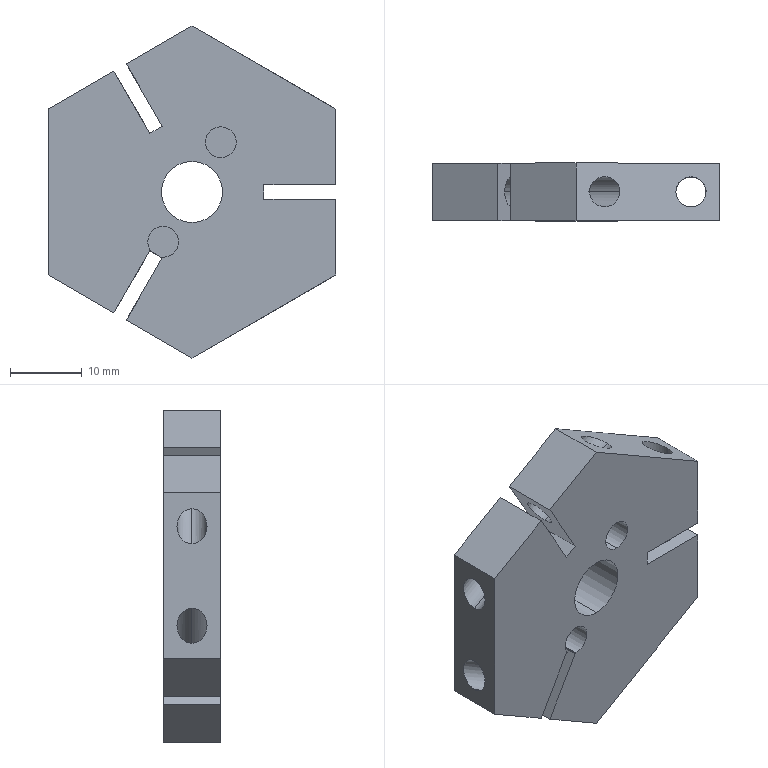Part | SolidWorks | features ICE 3, CirPattern 2, Cut 1, Extrusion 1 | 1 solid | 41 faces | box 40 x 8 x 46.188 mm | volume 8880 mm3 | plane 22 | cylinder 19 | commonest cylinder face diameters 4.2 x12 4.3 x5 8.5 x2
STEP:
#1=CARTESIAN_POINT('',(-4.,0.,-9.078));
#2=VERTEX_POINT('',#1);
#3=CARTESIAN_POINT('',(-4.317,0.,-9.055));
#4=VERTEX_POINT('',#3);
#5=CARTESIAN_POINT('',(-4.,0.,-6.928));
#6=DIRECTION('',(0.,1.,0.));
#7=DIRECTION('',(0.,0.,1.));
#8=AXIS2_PLACEMENT_3D('',#5,#6,#7);
#9=CIRCLE('',#8,2.15);
#10=EDGE_CURVE('',#2,#4,#9,.T.);
#11=ORIENTED_EDGE('',*,*,#10,.F.);
#12=CARTESIAN_POINT('',(-4.,7.,-9.078));
#13=VERTEX_POINT('',#12);
#14=CARTESIAN_POINT('',(-4.,-3.,-9.078));
#15=DIRECTION('',(0.,1.,0.));
#16=VECTOR('',#15,1000.);
#17=LINE('',#14,#16);
#18=EDGE_CURVE('',#2,#13,#17,.T.);
#19=ORIENTED_EDGE('',*,*,#18,.T.);
#20=CARTESIAN_POINT('',(-4.317,7.,-9.055));
#21=VERTEX_POINT('',#20);
#22=CARTESIAN_POINT('',(-4.,7.,-6.928));
#23=DIRECTION('',(0.,1.,0.));
#24=DIRECTION('',(0.,0.,1.));
#25=AXIS2_PLACEMENT_3D('',#22,#23,#24);
#26=CIRCLE('',#25,2.15);
#27=EDGE_CURVE('',#13,#21,#26,.T.);
#28=ORIENTED_EDGE('',*,*,#27,.T.);
#29=CARTESIAN_POINT('',(-4.317,-3.,-9.055));
#30=DIRECTION('',(0.,1.,0.));
#31=VECTOR('',#30,1000.);
#32=LINE('',#29,#31);
#33=EDGE_CURVE('',#4,#21,#32,.T.);
#34=ORIENTED_EDGE('',*,*,#33,.F.);
#35=EDGE_LOOP('',(#11,#19,#28,#34));
#36=FACE_OUTER_BOUND('',#35,.T.);
#37=CARTESIAN_POINT('',(-4.,-3.,-6.928));
#38=DIRECTION('',(0.,1.,0.));
#39=DIRECTION('',(0.,0.,1.));
#40=AXIS2_PLACEMENT_3D('',#37,#38,#39);
#41=CYLINDRICAL_SURFACE('',#40,2.15);
#42=ADVANCED_FACE('',(#36),#41,.F.);
#43=ORIENTED_EDGE('',*,*,#18,.F.);
#44=CARTESIAN_POINT('',(-4.,0.,-4.778));
#45=VERTEX_POINT('',#44);
#46=CARTESIAN_POINT('',(-4.,0.,-6.928));
#47=DIRECTION('',(0.,1.,0.));
#48=DIRECTION('',(0.,0.,1.));
#49=AXIS2_PLACEMENT_3D('',#46,#47,#48);
#50=CIRCLE('',#49,2.15);
#51=EDGE_CURVE('',#45,#2,#50,.T.);
#52=ORIENTED_EDGE('',*,*,#51,.F.);
#53=CARTESIAN_POINT('',(-4.,7.,-4.778));
#54=VERTEX_POINT('',#53);
#55=CARTESIAN_POINT('',(-4.,-3.,-4.778));
#56=DIRECTION('',(0.,1.,0.));
#57=VECTOR('',#56,1000.);
#58=LINE('',#55,#57);
#59=EDGE_CURVE('',#45,#54,#58,.T.);
#60=ORIENTED_EDGE('',*,*,#59,.T.);
#61=CARTESIAN_POINT('',(-4.,7.,-6.928));
#62=DIRECTION('',(0.,1.,0.));
#63=DIRECTION('',(0.,0.,1.));
#64=AXIS2_PLACEMENT_3D('',#61,#62,#63);
#65=CIRCLE('',#64,2.15);
#66=EDGE_CURVE('',#54,#13,#65,.T.);
#67=ORIENTED_EDGE('',*,*,#66,.T.);
#68=EDGE_LOOP('',(#43,#52,#60,#67));
#69=FACE_OUTER_BOUND('',#68,.T.);
#70=CARTESIAN_POINT('',(-4.,-3.,-6.928));
#71=DIRECTION('',(0.,1.,0.));
#72=DIRECTION('',(0.,0.,1.));
#73=AXIS2_PLACEMENT_3D('',#70,#71,#72);
#74=CYLINDRICAL_SURFACE('',#73,2.15);
#75=ADVANCED_FACE('',(#69),#74,.F.);
#76=CARTESIAN_POINT('',(4.,0.,4.778));
#77=VERTEX_POINT('',#76);
#78=CARTESIAN_POINT('',(4.,0.,9.078));
#79=VERTEX_POINT('',#78);
#80=CARTESIAN_POINT('',(4.,0.,6.928));
#81=DIRECTION('',(0.,1.,0.));
#82=DIRECTION('',(0.,0.,1.));
#83=AXIS2_PLACEMENT_3D('',#80,#81,#82);
#84=CIRCLE('',#83,2.15);
#85=EDGE_CURVE('',#77,#79,#84,.T.);
#86=ORIENTED_EDGE('',*,*,#85,.F.);
#87=CARTESIAN_POINT('',(4.,7.,4.778));
#88=VERTEX_POINT('',#87);
#89=CARTESIAN_POINT('',(4.,-3.,4.778));
#90=DIRECTION('',(0.,1.,0.));
#91=VECTOR('',#90,1000.);
#92=LINE('',#89,#91);
#93=EDGE_CURVE('',#77,#88,#92,.T.);
#94=ORIENTED_EDGE('',*,*,#93,.T.);
#95=CARTESIAN_POINT('',(4.,7.,9.078));
#96=VERTEX_POINT('',#95);
#97=CARTESIAN_POINT('',(4.,7.,6.928));
#98=DIRECTION('',(0.,1.,0.));
#99=DIRECTION('',(0.,0.,1.));
#100=AXIS2_PLACEMENT_3D('',#97,#98,#99);
#101=CIRCLE('',#100,2.15);
#102=EDGE_CURVE('',#88,#96,#101,.T.);
#103=ORIENTED_EDGE('',*,*,#102,.T.);
#104=CARTESIAN_POINT('',(4.,-3.,9.078));
#105=DIRECTION('',(0.,1.,0.));
#106=VECTOR('',#105,1000.);
#107=LINE('',#104,#106);
#108=EDGE_CURVE('',#79,#96,#107,.T.);
#109=ORIENTED_EDGE('',*,*,#108,.F.);
#110=EDGE_LOOP('',(#86,#94,#103,#109));
#111=FACE_OUTER_BOUND('',#110,.T.);
#112=CARTESIAN_POINT('',(4.,-3.,6.928));
#113=DIRECTION('',(0.,1.,0.));
#114=DIRECTION('',(0.,0.,1.));
#115=AXIS2_PLACEMENT_3D('',#112,#113,#114);
#116=CYLINDRICAL_SURFACE('',#115,2.15);
#117=ADVANCED_FACE('',(#111),#116,.F.);
#118=CARTESIAN_POINT('',(-6.084,4.,-12.538));
#119=VERTEX_POINT('',#118);
#120=CARTESIAN_POINT('',(-8.184,4.,-16.175));
#121=VERTEX_POINT('',#120);
#122=CARTESIAN_POINT('',(-7.134,4.,-14.356));
#123=DIRECTION('',(0.866,0.,-0.5));
#124=DIRECTION('',(-0.5,0.,-0.866));
#125=AXIS2_PLACEMENT_3D('',#122,#123,#124);
#126=CIRCLE('',#125,2.1);
#127=EDGE_CURVE('',#119,#121,#126,.T.);
#128=ORIENTED_EDGE('',*,*,#127,.F.);
#129=CARTESIAN_POINT('',(6.1,4.,-19.572));
#130=VERTEX_POINT('',#129);
#131=CARTESIAN_POINT('',(-31.95,4.,2.396));
#132=DIRECTION('',(0.866,0.,-0.5));
#133=VECTOR('',#132,1000.);
#134=LINE('',#131,#133);
#135=EDGE_CURVE('',#119,#130,#134,.T.);
#136=ORIENTED_EDGE('',*,*,#135,.T.);
#137=CARTESIAN_POINT('',(1.9,4.,-21.997));
#138=VERTEX_POINT('',#137);
#139=CARTESIAN_POINT('',(1.9,4.,-21.997));
#140=CARTESIAN_POINT('',(1.9,-0.2,-21.997));
#141=CARTESIAN_POINT('',(6.1,-0.2,-19.572));
#142=CARTESIAN_POINT('',(6.1,4.,-19.572));
#143=(BOUNDED_CURVE()B_SPLINE_CURVE(3,(#139,#140,#141,#142),.UNSPECIFIED.,.F.,.F.)B_SPLINE_CURVE_WITH_KNOTS((4,4),(3.142,6.283),.UNSPECIFIED.)CURVE()GEOMETRIC_REPRESENTATION_ITEM()RATIONAL_B_SPLINE_CURVE((1.,0.3333,0.3333,1.))REPRESENTATION_ITEM(''));
#144=EDGE_CURVE('',#138,#130,#143,.T.);
#145=ORIENTED_EDGE('',*,*,#144,.F.);
#146=CARTESIAN_POINT('',(-34.05,4.,-1.241));
#147=DIRECTION('',(0.866,0.,-0.5));
#148=VECTOR('',#147,1000.);
#149=LINE('',#146,#148);
#150=EDGE_CURVE('',#121,#138,#149,.T.);
#151=ORIENTED_EDGE('',*,*,#150,.F.);
#152=EDGE_LOOP('',(#128,#136,#145,#151));
#153=FACE_OUTER_BOUND('',#152,.T.);
#154=CARTESIAN_POINT('',(-33.,4.,0.5774));
#155=DIRECTION('',(0.866,0.,-0.5));
#156=DIRECTION('',(-0.5,0.,-0.866));
#157=AXIS2_PLACEMENT_3D('',#154,#155,#156);
#158=CYLINDRICAL_SURFACE('',#157,2.1);
#159=ADVANCED_FACE('',(#153),#158,.F.);
#160=CARTESIAN_POINT('',(-20.,4.,-4.503));
#161=VERTEX_POINT('',#160);
#162=CARTESIAN_POINT('',(-20.,4.,-9.353));
#163=VERTEX_POINT('',#162);
#164=CARTESIAN_POINT('',(-20.,4.,-4.503));
#165=CARTESIAN_POINT('',(-20.,-0.2,-4.503));
#166=CARTESIAN_POINT('',(-20.,-0.2,-9.353));
#167=CARTESIAN_POINT('',(-20.,4.,-9.353));
#168=(BOUNDED_CURVE()B_SPLINE_CURVE(3,(#164,#165,#166,#167),.UNSPECIFIED.,.F.,.F.)B_SPLINE_CURVE_WITH_KNOTS((4,4),(3.142,6.283),.UNSPECIFIED.)CURVE()GEOMETRIC_REPRESENTATION_ITEM()RATIONAL_B_SPLINE_CURVE((1.,0.3333,0.3333,1.))REPRESENTATION_ITEM(''));
#169=EDGE_CURVE('',#161,#163,#168,.T.);
#170=ORIENTED_EDGE('',*,*,#169,.F.);
#171=CARTESIAN_POINT('',(-7.816,4.,-11.538));
#172=VERTEX_POINT('',#171);
#173=CARTESIAN_POINT('',(-31.95,4.,2.396));
#174=DIRECTION('',(0.866,0.,-0.5));
#175=VECTOR('',#174,1000.);
#176=LINE('',#173,#175);
#177=EDGE_CURVE('',#161,#172,#176,.T.);
#178=ORIENTED_EDGE('',*,*,#177,.T.);
#179=CARTESIAN_POINT('',(-9.916,4.,-15.175));
#180=VERTEX_POINT('',#179);
#181=CARTESIAN_POINT('',(-8.866,4.,-13.356));
#182=DIRECTION('',(-0.866,0.,0.5));
#183=DIRECTION('',(0.5,0.,0.866));
#184=AXIS2_PLACEMENT_3D('',#181,#182,#183);
#185=CIRCLE('',#184,2.1);
#186=EDGE_CURVE('',#180,#172,#185,.T.);
#187=ORIENTED_EDGE('',*,*,#186,.F.);
#188=CARTESIAN_POINT('',(-34.05,4.,-1.241));
#189=DIRECTION('',(0.866,0.,-0.5));
#190=VECTOR('',#189,1000.);
#191=LINE('',#188,#190);
#192=EDGE_CURVE('',#163,#180,#191,.T.);
#193=ORIENTED_EDGE('',*,*,#192,.F.);
#194=EDGE_LOOP('',(#170,#178,#187,#193));
#195=FACE_OUTER_BOUND('',#194,.T.);
#196=CARTESIAN_POINT('',(-33.,4.,0.5774));
#197=DIRECTION('',(0.866,0.,-0.5));
#198=DIRECTION('',(-0.5,0.,-0.866));
#199=AXIS2_PLACEMENT_3D('',#196,#197,#198);
#200=CYLINDRICAL_SURFACE('',#199,2.1);
#201=ADVANCED_FACE('',(#195),#200,.F.);
#202=CARTESIAN_POINT('',(-7.816,4.,11.538));
#203=VERTEX_POINT('',#202);
#204=CARTESIAN_POINT('',(-9.916,4.,15.175));
#205=VERTEX_POINT('',#204);
#206=CARTESIAN_POINT('',(-8.866,4.,13.356));
#207=DIRECTION('',(-0.866,0.,-0.5));
#208=DIRECTION('',(-0.5,0.,0.866));
#209=AXIS2_PLACEMENT_3D('',#206,#207,#208);
#210=CIRCLE('',#209,2.1);
#211=EDGE_CURVE('',#203,#205,#210,.T.);
#212=ORIENTED_EDGE('',*,*,#211,.F.);
#213=CARTESIAN_POINT('',(-20.,4.,4.503));
#214=VERTEX_POINT('',#213);
#215=CARTESIAN_POINT('',(18.05,4.,26.472));
#216=DIRECTION('',(-0.866,0.,-0.5));
#217=VECTOR('',#216,1000.);
#218=LINE('',#215,#217);
#219=EDGE_CURVE('',#203,#214,#218,.T.);
#220=ORIENTED_EDGE('',*,*,#219,.T.);
#221=CARTESIAN_POINT('',(-20.,4.,9.353));
#222=VERTEX_POINT('',#221);
#223=CARTESIAN_POINT('',(-20.,4.,9.353));
#224=CARTESIAN_POINT('',(-20.,-0.2,9.353));
#225=CARTESIAN_POINT('',(-20.,-0.2,4.503));
#226=CARTESIAN_POINT('',(-20.,4.,4.503));
#227=(BOUNDED_CURVE()B_SPLINE_CURVE(3,(#223,#224,#225,#226),.UNSPECIFIED.,.F.,.F.)B_SPLINE_CURVE_WITH_KNOTS((4,4),(3.142,6.283),.UNSPECIFIED.)CURVE()GEOMETRIC_REPRESENTATION_ITEM()RATIONAL_B_SPLINE_CURVE((1.,0.3333,0.3333,1.))REPRESENTATION_ITEM(''));
#228=EDGE_CURVE('',#222,#214,#227,.T.);
#229=ORIENTED_EDGE('',*,*,#228,.F.);
#230=CARTESIAN_POINT('',(15.95,4.,30.109));
#231=DIRECTION('',(-0.866,0.,-0.5));
#232=VECTOR('',#231,1000.);
#233=LINE('',#230,#232);
#234=EDGE_CURVE('',#205,#222,#233,.T.);
#235=ORIENTED_EDGE('',*,*,#234,.F.);
#236=EDGE_LOOP('',(#212,#220,#229,#235));
#237=FACE_OUTER_BOUND('',#236,.T.);
#238=CARTESIAN_POINT('',(17.,4.,28.29));
#239=DIRECTION('',(-0.866,0.,-0.5));
#240=DIRECTION('',(-0.5,0.,0.866));
#241=AXIS2_PLACEMENT_3D('',#238,#239,#240);
#242=CYLINDRICAL_SURFACE('',#241,2.1);
#243=ADVANCED_FACE('',(#237),#242,.F.);
#244=CARTESIAN_POINT('',(6.1,4.,19.572));
#245=VERTEX_POINT('',#244);
#246=CARTESIAN_POINT('',(1.9,4.,21.997));
#247=VERTEX_POINT('',#246);
#248=CARTESIAN_POINT('',(6.1,4.,19.572));
#249=CARTESIAN_POINT('',(6.1,-0.2,19.572));
#250=CARTESIAN_POINT('',(1.9,-0.2,21.997));
#251=CARTESIAN_POINT('',(1.9,4.,21.997));
#252=(BOUNDED_CURVE()B_SPLINE_CURVE(3,(#248,#249,#250,#251),.UNSPECIFIED.,.F.,.F.)B_SPLINE_CURVE_WITH_KNOTS((4,4),(3.142,6.283),.UNSPECIFIED.)CURVE()GEOMETRIC_REPRESENTATION_ITEM()RATIONAL_B_SPLINE_CURVE((1.,0.3333,0.3333,1.))REPRESENTATION_ITEM(''));
#253=EDGE_CURVE('',#245,#247,#252,.T.);
#254=ORIENTED_EDGE('',*,*,#253,.F.);
#255=CARTESIAN_POINT('',(-6.084,4.,12.538));
#256=VERTEX_POINT('',#255);
#257=CARTESIAN_POINT('',(18.05,4.,26.472));
#258=DIRECTION('',(-0.866,0.,-0.5));
#259=VECTOR('',#258,1000.);
#260=LINE('',#257,#259);
#261=EDGE_CURVE('',#245,#256,#260,.T.);
#262=ORIENTED_EDGE('',*,*,#261,.T.);
#263=CARTESIAN_POINT('',(-8.184,4.,16.175));
#264=VERTEX_POINT('',#263);
#265=CARTESIAN_POINT('',(-7.134,4.,14.356));
#266=DIRECTION('',(0.866,0.,0.5));
#267=DIRECTION('',(0.5,0.,-0.866));
#268=AXIS2_PLACEMENT_3D('',#265,#266,#267);
#269=CIRCLE('',#268,2.1);
#270=EDGE_CURVE('',#264,#256,#269,.T.);
#271=ORIENTED_EDGE('',*,*,#270,.F.);
#272=CARTESIAN_POINT('',(15.95,4.,30.109));
#273=DIRECTION('',(-0.866,0.,-0.5));
#274=VECTOR('',#273,1000.);
#275=LINE('',#272,#274);
#276=EDGE_CURVE('',#247,#264,#275,.T.);
#277=ORIENTED_EDGE('',*,*,#276,.F.);
#278=EDGE_LOOP('',(#254,#262,#271,#277));
#279=FACE_OUTER_BOUND('',#278,.T.);
#280=CARTESIAN_POINT('',(17.,4.,28.29));
#281=DIRECTION('',(-0.866,0.,-0.5));
#282=DIRECTION('',(-0.5,0.,0.866));
#283=AXIS2_PLACEMENT_3D('',#280,#281,#282);
#284=CYLINDRICAL_SURFACE('',#283,2.1);
#285=ADVANCED_FACE('',(#279),#284,.F.);
#286=CARTESIAN_POINT('',(13.9,4.,1.));
#287=VERTEX_POINT('',#286);
#288=CARTESIAN_POINT('',(18.1,4.,1.));
#289=VERTEX_POINT('',#288);
#290=CARTESIAN_POINT('',(16.,4.,1.));
#291=DIRECTION('',(0.,0.,1.));
#292=DIRECTION('',(1.,0.,0.));
#293=AXIS2_PLACEMENT_3D('',#290,#291,#292);
#294=CIRCLE('',#293,2.1);
#295=EDGE_CURVE('',#287,#289,#294,.T.);
#296=ORIENTED_EDGE('',*,*,#295,.F.);
#297=CARTESIAN_POINT('',(13.9,4.,15.069));
#298=VERTEX_POINT('',#297);
#299=CARTESIAN_POINT('',(13.9,4.,-23.094));
#300=DIRECTION('',(0.,0.,1.));
#301=VECTOR('',#300,1000.);
#302=LINE('',#299,#301);
#303=EDGE_CURVE('',#287,#298,#302,.T.);
#304=ORIENTED_EDGE('',*,*,#303,.T.);
#305=CARTESIAN_POINT('',(18.1,4.,12.644));
#306=VERTEX_POINT('',#305);
#307=CARTESIAN_POINT('',(18.1,4.,12.644));
#308=CARTESIAN_POINT('',(18.1,-0.2,12.644));
#309=CARTESIAN_POINT('',(13.9,-0.2,15.069));
#310=CARTESIAN_POINT('',(13.9,4.,15.069));
#311=(BOUNDED_CURVE()B_SPLINE_CURVE(3,(#307,#308,#309,#310),.UNSPECIFIED.,.F.,.F.)B_SPLINE_CURVE_WITH_KNOTS((4,4),(3.142,6.283),.UNSPECIFIED.)CURVE()GEOMETRIC_REPRESENTATION_ITEM()RATIONAL_B_SPLINE_CURVE((1.,0.3333,0.3333,1.))REPRESENTATION_ITEM(''));
#312=EDGE_CURVE('',#306,#298,#311,.T.);
#313=ORIENTED_EDGE('',*,*,#312,.F.);
#314=CARTESIAN_POINT('',(18.1,4.,-23.094));
#315=DIRECTION('',(0.,0.,1.));
#316=VECTOR('',#315,1000.);
#317=LINE('',#314,#316);
#318=EDGE_CURVE('',#289,#306,#317,.T.);
#319=ORIENTED_EDGE('',*,*,#318,.F.);
#320=EDGE_LOOP('',(#296,#304,#313,#319));
#321=FACE_OUTER_BOUND('',#320,.T.);
#322=CARTESIAN_POINT('',(16.,4.,-23.094));
#323=DIRECTION('',(0.,0.,1.));
#324=DIRECTION('',(1.,0.,0.));
#325=AXIS2_PLACEMENT_3D('',#322,#323,#324);
#326=CYLINDRICAL_SURFACE('',#325,2.1);
#327=ADVANCED_FACE('',(#321),#326,.F.);
#328=CARTESIAN_POINT('',(13.9,4.,-15.069));
#329=VERTEX_POINT('',#328);
#330=CARTESIAN_POINT('',(18.1,4.,-12.644));
#331=VERTEX_POINT('',#330);
#332=CARTESIAN_POINT('',(13.9,4.,-15.069));
#333=CARTESIAN_POINT('',(13.9,-0.2,-15.069));
#334=CARTESIAN_POINT('',(18.1,-0.2,-12.644));
#335=CARTESIAN_POINT('',(18.1,4.,-12.644));
#336=(BOUNDED_CURVE()B_SPLINE_CURVE(3,(#332,#333,#334,#335),.UNSPECIFIED.,.F.,.F.)B_SPLINE_CURVE_WITH_KNOTS((4,4),(3.142,6.283),.UNSPECIFIED.)CURVE()GEOMETRIC_REPRESENTATION_ITEM()RATIONAL_B_SPLINE_CURVE((1.,0.3333,0.3333,1.))REPRESENTATION_ITEM(''));
#337=EDGE_CURVE('',#329,#331,#336,.T.);
#338=ORIENTED_EDGE('',*,*,#337,.F.);
#339=CARTESIAN_POINT('',(13.9,4.,-1.));
#340=VERTEX_POINT('',#339);
#341=CARTESIAN_POINT('',(13.9,4.,-23.094));
#342=DIRECTION('',(0.,0.,1.));
#343=VECTOR('',#342,1000.);
#344=LINE('',#341,#343);
#345=EDGE_CURVE('',#329,#340,#344,.T.);
#346=ORIENTED_EDGE('',*,*,#345,.T.);
#347=CARTESIAN_POINT('',(18.1,4.,-1.));
#348=VERTEX_POINT('',#347);
#349=CARTESIAN_POINT('',(16.,4.,-1.));
#350=DIRECTION('',(0.,0.,-1.));
#351=DIRECTION('',(-1.,0.,0.));
#352=AXIS2_PLACEMENT_3D('',#349,#350,#351);
#353=CIRCLE('',#352,2.1);
#354=EDGE_CURVE('',#348,#340,#353,.T.);
#355=ORIENTED_EDGE('',*,*,#354,.F.);
#356=CARTESIAN_POINT('',(18.1,4.,-23.094));
#357=DIRECTION('',(0.,0.,1.));
#358=VECTOR('',#357,1000.);
#359=LINE('',#356,#358);
#360=EDGE_CURVE('',#331,#348,#359,.T.);
#361=ORIENTED_EDGE('',*,*,#360,.F.);
#362=EDGE_LOOP('',(#338,#346,#355,#361));
#363=FACE_OUTER_BOUND('',#362,.T.);
#364=CARTESIAN_POINT('',(16.,4.,-23.094));
#365=DIRECTION('',(0.,0.,1.));
#366=DIRECTION('',(1.,0.,0.));
#367=AXIS2_PLACEMENT_3D('',#364,#365,#366);
#368=CYLINDRICAL_SURFACE('',#367,2.1);
#369=ADVANCED_FACE('',(#363),#368,.F.);
#370=CARTESIAN_POINT('',(0.,0.,-4.25));
#371=VERTEX_POINT('',#370);
#372=CARTESIAN_POINT('',(0.,0.,4.25));
#373=VERTEX_POINT('',#372);
#374=CARTESIAN_POINT('',(0.,0.,0.));
#375=DIRECTION('',(0.,1.,0.));
#376=DIRECTION('',(0.,0.,1.));
#377=AXIS2_PLACEMENT_3D('',#374,#375,#376);
#378=CIRCLE('',#377,4.25);
#379=EDGE_CURVE('',#371,#373,#378,.T.);
#380=ORIENTED_EDGE('',*,*,#379,.F.);
#381=CARTESIAN_POINT('',(0.,8.,-4.25));
#382=VERTEX_POINT('',#381);
#383=CARTESIAN_POINT('',(0.,-2.,-4.25));
#384=DIRECTION('',(0.,1.,0.));
#385=VECTOR('',#384,1000.);
#386=LINE('',#383,#385);
#387=EDGE_CURVE('',#371,#382,#386,.T.);
#388=ORIENTED_EDGE('',*,*,#387,.T.);
#389=CARTESIAN_POINT('',(0.,8.,4.25));
#390=VERTEX_POINT('',#389);
#391=CARTESIAN_POINT('',(0.,8.,0.));
#392=DIRECTION('',(0.,1.,0.));
#393=DIRECTION('',(0.,0.,1.));
#394=AXIS2_PLACEMENT_3D('',#391,#392,#393);
#395=CIRCLE('',#394,4.25);
#396=EDGE_CURVE('',#382,#390,#395,.T.);
#397=ORIENTED_EDGE('',*,*,#396,.T.);
#398=CARTESIAN_POINT('',(0.,-2.,4.25));
#399=DIRECTION('',(0.,1.,0.));
#400=VECTOR('',#399,1000.);
#401=LINE('',#398,#400);
#402=EDGE_CURVE('',#373,#390,#401,.T.);
#403=ORIENTED_EDGE('',*,*,#402,.F.);
#404=EDGE_LOOP('',(#380,#388,#397,#403));
#405=FACE_OUTER_BOUND('',#404,.T.);
#406=CARTESIAN_POINT('',(0.,-2.,0.));
#407=DIRECTION('',(0.,1.,0.));
#408=DIRECTION('',(0.,0.,1.));
#409=AXIS2_PLACEMENT_3D('',#406,#407,#408);
#410=CYLINDRICAL_SURFACE('',#409,4.25);
#411=ADVANCED_FACE('',(#405),#410,.F.);
#412=CARTESIAN_POINT('',(20.,0.,11.547));
#413=VERTEX_POINT('',#412);
#414=CARTESIAN_POINT('',(20.,0.,1.));
#415=VERTEX_POINT('',#414);
#416=CARTESIAN_POINT('',(20.,0.,11.547));
#417=DIRECTION('',(0.,0.,-1.));
#418=VECTOR('',#417,1000.);
#419=LINE('',#416,#418);
#420=EDGE_CURVE('',#413,#415,#419,.T.);
#421=ORIENTED_EDGE('',*,*,#420,.T.);
#422=CARTESIAN_POINT('',(20.,8.,1.));
#423=VERTEX_POINT('',#422);
#424=CARTESIAN_POINT('',(20.,-2.,1.));
#425=DIRECTION('',(0.,1.,0.));
#426=VECTOR('',#425,1000.);
#427=LINE('',#424,#426);
#428=EDGE_CURVE('',#415,#423,#427,.T.);
#429=ORIENTED_EDGE('',*,*,#428,.T.);
#430=CARTESIAN_POINT('',(20.,8.,11.547));
#431=VERTEX_POINT('',#430);
#432=CARTESIAN_POINT('',(20.,8.,11.547));
#433=DIRECTION('',(0.,0.,-1.));
#434=VECTOR('',#433,1000.);
#435=LINE('',#432,#434);
#436=EDGE_CURVE('',#431,#423,#435,.T.);
#437=ORIENTED_EDGE('',*,*,#436,.F.);
#438=CARTESIAN_POINT('',(20.,8.,11.547));
#439=DIRECTION('',(0.,-1.,0.));
#440=VECTOR('',#439,1000.);
#441=LINE('',#438,#440);
#442=EDGE_CURVE('',#431,#413,#441,.T.);
#443=ORIENTED_EDGE('',*,*,#442,.T.);
#444=EDGE_LOOP('',(#421,#429,#437,#443));
#445=FACE_OUTER_BOUND('',#444,.T.);
#446=CARTESIAN_POINT('',(20.,8.,11.547));
#447=DIRECTION('',(-1.,0.,0.));
#448=DIRECTION('',(0.,0.,1.));
#449=AXIS2_PLACEMENT_3D('',#446,#447,#448);
#450=PLANE('',#449);
#451=ADVANCED_FACE('',(#445),#450,.F.);
#452=CARTESIAN_POINT('',(-20.,0.,11.547));
#453=VERTEX_POINT('',#452);
#454=CARTESIAN_POINT('',(-10.866,0.,16.821));
#455=VERTEX_POINT('',#454);
#456=CARTESIAN_POINT('',(-20.,0.,11.547));
#457=DIRECTION('',(0.866,0.,0.5));
#458=VECTOR('',#457,1000.);
#459=LINE('',#456,#458);
#460=EDGE_CURVE('',#453,#455,#459,.T.);
#461=ORIENTED_EDGE('',*,*,#460,.T.);
#462=CARTESIAN_POINT('',(-10.866,8.,16.821));
#463=VERTEX_POINT('',#462);
#464=CARTESIAN_POINT('',(-10.866,-2.,16.821));
#465=DIRECTION('',(0.,1.,0.));
#466=VECTOR('',#465,1000.);
#467=LINE('',#464,#466);
#468=EDGE_CURVE('',#455,#463,#467,.T.);
#469=ORIENTED_EDGE('',*,*,#468,.T.);
#470=CARTESIAN_POINT('',(-20.,8.,11.547));
#471=VERTEX_POINT('',#470);
#472=CARTESIAN_POINT('',(-20.,8.,11.547));
#473=DIRECTION('',(0.866,0.,0.5));
#474=VECTOR('',#473,1000.);
#475=LINE('',#472,#474);
#476=EDGE_CURVE('',#471,#463,#475,.T.);
#477=ORIENTED_EDGE('',*,*,#476,.F.);
#478=CARTESIAN_POINT('',(-20.,8.,11.547));
#479=DIRECTION('',(0.,-1.,0.));
#480=VECTOR('',#479,1000.);
#481=LINE('',#478,#480);
#482=EDGE_CURVE('',#471,#453,#481,.T.);
#483=ORIENTED_EDGE('',*,*,#482,.T.);
#484=EDGE_LOOP('',(#461,#469,#477,#483));
#485=FACE_OUTER_BOUND('',#484,.T.);
#486=CARTESIAN_POINT('',(-20.,8.,11.547));
#487=DIRECTION('',(0.5,0.,-0.866));
#488=DIRECTION('',(-0.866,0.,-0.5));
#489=AXIS2_PLACEMENT_3D('',#486,#487,#488);
#490=PLANE('',#489);
#491=ADVANCED_FACE('',(#485),#490,.F.);
#492=CARTESIAN_POINT('',(0.,0.,-23.094));
#493=VERTEX_POINT('',#492);
#494=CARTESIAN_POINT('',(-9.134,0.,-17.821));
#495=VERTEX_POINT('',#494);
#496=CARTESIAN_POINT('',(0.,0.,-23.094));
#497=DIRECTION('',(-0.866,0.,0.5));
#498=VECTOR('',#497,1000.);
#499=LINE('',#496,#498);
#500=EDGE_CURVE('',#493,#495,#499,.T.);
#501=ORIENTED_EDGE('',*,*,#500,.T.);
#502=CARTESIAN_POINT('',(-9.134,8.,-17.821));
#503=VERTEX_POINT('',#502);
#504=CARTESIAN_POINT('',(-9.134,-2.,-17.821));
#505=DIRECTION('',(0.,1.,0.));
#506=VECTOR('',#505,1000.);
#507=LINE('',#504,#506);
#508=EDGE_CURVE('',#495,#503,#507,.T.);
#509=ORIENTED_EDGE('',*,*,#508,.T.);
#510=CARTESIAN_POINT('',(0.,8.,-23.094));
#511=VERTEX_POINT('',#510);
#512=CARTESIAN_POINT('',(0.,8.,-23.094));
#513=DIRECTION('',(-0.866,0.,0.5));
#514=VECTOR('',#513,1000.);
#515=LINE('',#512,#514);
#516=EDGE_CURVE('',#511,#503,#515,.T.);
#517=ORIENTED_EDGE('',*,*,#516,.F.);
#518=CARTESIAN_POINT('',(0.,8.,-23.094));
#519=DIRECTION('',(0.,-1.,0.));
#520=VECTOR('',#519,1000.);
#521=LINE('',#518,#520);
#522=EDGE_CURVE('',#511,#493,#521,.T.);
#523=ORIENTED_EDGE('',*,*,#522,.T.);
#524=EDGE_LOOP('',(#501,#509,#517,#523));
#525=FACE_OUTER_BOUND('',#524,.T.);
#526=CARTESIAN_POINT('',(0.,8.,-23.094));
#527=DIRECTION('',(0.5,0.,0.866));
#528=DIRECTION('',(0.866,0.,-0.5));
#529=AXIS2_PLACEMENT_3D('',#526,#527,#528);
#530=PLANE('',#529);
#531=ADVANCED_FACE('',(#525),#530,.F.);
#532=ORIENTED_EDGE('',*,*,#144,.T.);
#533=CARTESIAN_POINT('',(6.1,4.,-19.572));
#534=CARTESIAN_POINT('',(6.1,8.2,-19.572));
#535=CARTESIAN_POINT('',(1.9,8.2,-21.997));
#536=CARTESIAN_POINT('',(1.9,4.,-21.997));
#537=(BOUNDED_CURVE()B_SPLINE_CURVE(3,(#533,#534,#535,#536),.UNSPECIFIED.,.F.,.F.)B_SPLINE_CURVE_WITH_KNOTS((4,4),(0.,3.142),.UNSPECIFIED.)CURVE()GEOMETRIC_REPRESENTATION_ITEM()RATIONAL_B_SPLINE_CURVE((1.,0.3333,0.3333,1.))REPRESENTATION_ITEM(''));
#538=EDGE_CURVE('',#130,#138,#537,.T.);
#539=ORIENTED_EDGE('',*,*,#538,.T.);
#540=EDGE_LOOP('',(#532,#539));
#541=FACE_BOUND('',#540,.T.);
#542=CARTESIAN_POINT('',(18.1,4.,-12.644));
#543=CARTESIAN_POINT('',(18.1,8.2,-12.644));
#544=CARTESIAN_POINT('',(13.9,8.2,-15.069));
#545=CARTESIAN_POINT('',(13.9,4.,-15.069));
#546=(BOUNDED_CURVE()B_SPLINE_CURVE(3,(#542,#543,#544,#545),.UNSPECIFIED.,.F.,.F.)B_SPLINE_CURVE_WITH_KNOTS((4,4),(0.,3.142),.UNSPECIFIED.)CURVE()GEOMETRIC_REPRESENTATION_ITEM()RATIONAL_B_SPLINE_CURVE((1.,0.3333,0.3333,1.))REPRESENTATION_ITEM(''));
#547=EDGE_CURVE('',#331,#329,#546,.T.);
#548=ORIENTED_EDGE('',*,*,#547,.T.);
#549=ORIENTED_EDGE('',*,*,#337,.T.);
#550=EDGE_LOOP('',(#548,#549));
#551=FACE_BOUND('',#550,.T.);
#552=CARTESIAN_POINT('',(20.,0.,-11.547));
#553=VERTEX_POINT('',#552);
#554=CARTESIAN_POINT('',(20.,0.,-11.547));
#555=DIRECTION('',(-0.866,0.,-0.5));
#556=VECTOR('',#555,1000.);
#557=LINE('',#554,#556);
#558=EDGE_CURVE('',#553,#493,#557,.T.);
#559=ORIENTED_EDGE('',*,*,#558,.T.);
#560=ORIENTED_EDGE('',*,*,#522,.F.);
#561=CARTESIAN_POINT('',(20.,8.,-11.547));
#562=VERTEX_POINT('',#561);
#563=CARTESIAN_POINT('',(20.,8.,-11.547));
#564=DIRECTION('',(-0.866,0.,-0.5));
#565=VECTOR('',#564,1000.);
#566=LINE('',#563,#565);
#567=EDGE_CURVE('',#562,#511,#566,.T.);
#568=ORIENTED_EDGE('',*,*,#567,.F.);
#569=CARTESIAN_POINT('',(20.,8.,-11.547));
#570=DIRECTION('',(0.,-1.,0.));
#571=VECTOR('',#570,1000.);
#572=LINE('',#569,#571);
#573=EDGE_CURVE('',#562,#553,#572,.T.);
#574=ORIENTED_EDGE('',*,*,#573,.T.);
#575=EDGE_LOOP('',(#559,#560,#568,#574));
#576=FACE_OUTER_BOUND('',#575,.T.);
#577=CARTESIAN_POINT('',(20.,8.,-11.547));
#578=DIRECTION('',(-0.5,0.,0.866));
#579=DIRECTION('',(0.866,0.,0.5));
#580=AXIS2_PLACEMENT_3D('',#577,#578,#579);
#581=PLANE('',#580);
#582=ADVANCED_FACE('',(#541,#551,#576),#581,.F.);
#583=CARTESIAN_POINT('',(-10.866,8.,-16.821));
#584=VERTEX_POINT('',#583);
#585=CARTESIAN_POINT('',(-20.,8.,-11.547));
#586=VERTEX_POINT('',#585);
#587=CARTESIAN_POINT('',(0.,8.,-23.094));
#588=DIRECTION('',(-0.866,0.,0.5));
#589=VECTOR('',#588,1000.);
#590=LINE('',#587,#589);
#591=EDGE_CURVE('',#584,#586,#590,.T.);
#592=ORIENTED_EDGE('',*,*,#591,.F.);
#593=CARTESIAN_POINT('',(-10.866,0.,-16.821));
#594=VERTEX_POINT('',#593);
#595=CARTESIAN_POINT('',(-10.866,-2.,-16.821));
#596=DIRECTION('',(0.,1.,0.));
#597=VECTOR('',#596,1000.);
#598=LINE('',#595,#597);
#599=EDGE_CURVE('',#594,#584,#598,.T.);
#600=ORIENTED_EDGE('',*,*,#599,.F.);
#601=CARTESIAN_POINT('',(-20.,0.,-11.547));
#602=VERTEX_POINT('',#601);
#603=CARTESIAN_POINT('',(0.,0.,-23.094));
#604=DIRECTION('',(-0.866,0.,0.5));
#605=VECTOR('',#604,1000.);
#606=LINE('',#603,#605);
#607=EDGE_CURVE('',#594,#602,#606,.T.);
#608=ORIENTED_EDGE('',*,*,#607,.T.);
#609=CARTESIAN_POINT('',(-20.,8.,-11.547));
#610=DIRECTION('',(0.,-1.,0.));
#611=VECTOR('',#610,1000.);
#612=LINE('',#609,#611);
#613=EDGE_CURVE('',#586,#602,#612,.T.);
#614=ORIENTED_EDGE('',*,*,#613,.F.);
#615=EDGE_LOOP('',(#592,#600,#608,#614));
#616=FACE_OUTER_BOUND('',#615,.T.);
#617=CARTESIAN_POINT('',(0.,8.,-23.094));
#618=DIRECTION('',(0.5,0.,0.866));
#619=DIRECTION('',(0.866,0.,-0.5));
#620=AXIS2_PLACEMENT_3D('',#617,#618,#619);
#621=PLANE('',#620);
#622=ADVANCED_FACE('',(#616),#621,.F.);
#623=CARTESIAN_POINT('',(-20.,4.,-9.353));
#624=CARTESIAN_POINT('',(-20.,8.2,-9.353));
#625=CARTESIAN_POINT('',(-20.,8.2,-4.503));
#626=CARTESIAN_POINT('',(-20.,4.,-4.503));
#627=(BOUNDED_CURVE()B_SPLINE_CURVE(3,(#623,#624,#625,#626),.UNSPECIFIED.,.F.,.F.)B_SPLINE_CURVE_WITH_KNOTS((4,4),(0.,3.142),.UNSPECIFIED.)CURVE()GEOMETRIC_REPRESENTATION_ITEM()RATIONAL_B_SPLINE_CURVE((1.,0.3333,0.3333,1.))REPRESENTATION_ITEM(''));
#628=EDGE_CURVE('',#163,#161,#627,.T.);
#629=ORIENTED_EDGE('',*,*,#628,.T.);
#630=ORIENTED_EDGE('',*,*,#169,.T.);
#631=EDGE_LOOP('',(#629,#630));
#632=FACE_BOUND('',#631,.T.);
#633=ORIENTED_EDGE('',*,*,#228,.T.);
#634=CARTESIAN_POINT('',(-20.,4.,4.503));
#635=CARTESIAN_POINT('',(-20.,8.2,4.503));
#636=CARTESIAN_POINT('',(-20.,8.2,9.353));
#637=CARTESIAN_POINT('',(-20.,4.,9.353));
#638=(BOUNDED_CURVE()B_SPLINE_CURVE(3,(#634,#635,#636,#637),.UNSPECIFIED.,.F.,.F.)B_SPLINE_CURVE_WITH_KNOTS((4,4),(0.,3.142),.UNSPECIFIED.)CURVE()GEOMETRIC_REPRESENTATION_ITEM()RATIONAL_B_SPLINE_CURVE((1.,0.3333,0.3333,1.))REPRESENTATION_ITEM(''));
#639=EDGE_CURVE('',#214,#222,#638,.T.);
#640=ORIENTED_EDGE('',*,*,#639,.T.);
#641=EDGE_LOOP('',(#633,#640));
#642=FACE_BOUND('',#641,.T.);
#643=CARTESIAN_POINT('',(-20.,0.,-11.547));
#644=DIRECTION('',(0.,0.,1.));
#645=VECTOR('',#644,1000.);
#646=LINE('',#643,#645);
#647=EDGE_CURVE('',#602,#453,#646,.T.);
#648=ORIENTED_EDGE('',*,*,#647,.T.);
#649=ORIENTED_EDGE('',*,*,#482,.F.);
#650=CARTESIAN_POINT('',(-20.,8.,-11.547));
#651=DIRECTION('',(0.,0.,1.));
#652=VECTOR('',#651,1000.);
#653=LINE('',#650,#652);
#654=EDGE_CURVE('',#586,#471,#653,.T.);
#655=ORIENTED_EDGE('',*,*,#654,.F.);
#656=ORIENTED_EDGE('',*,*,#613,.T.);
#657=EDGE_LOOP('',(#648,#649,#655,#656));
#658=FACE_OUTER_BOUND('',#657,.T.);
#659=CARTESIAN_POINT('',(-20.,8.,-11.547));
#660=DIRECTION('',(1.,0.,0.));
#661=DIRECTION('',(0.,0.,-1.));
#662=AXIS2_PLACEMENT_3D('',#659,#660,#661);
#663=PLANE('',#662);
#664=ADVANCED_FACE('',(#632,#642,#658),#663,.F.);
#665=CARTESIAN_POINT('',(-9.134,8.,17.821));
#666=VERTEX_POINT('',#665);
#667=CARTESIAN_POINT('',(0.,8.,23.094));
#668=VERTEX_POINT('',#667);
#669=CARTESIAN_POINT('',(-20.,8.,11.547));
#670=DIRECTION('',(0.866,0.,0.5));
#671=VECTOR('',#670,1000.);
#672=LINE('',#669,#671);
#673=EDGE_CURVE('',#666,#668,#672,.T.);
#674=ORIENTED_EDGE('',*,*,#673,.F.);
#675=CARTESIAN_POINT('',(-9.134,0.,17.821));
#676=VERTEX_POINT('',#675);
#677=CARTESIAN_POINT('',(-9.134,-2.,17.821));
#678=DIRECTION('',(0.,1.,0.));
#679=VECTOR('',#678,1000.);
#680=LINE('',#677,#679);
#681=EDGE_CURVE('',#676,#666,#680,.T.);
#682=ORIENTED_EDGE('',*,*,#681,.F.);
#683=CARTESIAN_POINT('',(0.,0.,23.094));
#684=VERTEX_POINT('',#683);
#685=CARTESIAN_POINT('',(-20.,0.,11.547));
#686=DIRECTION('',(0.866,0.,0.5));
#687=VECTOR('',#686,1000.);
#688=LINE('',#685,#687);
#689=EDGE_CURVE('',#676,#684,#688,.T.);
#690=ORIENTED_EDGE('',*,*,#689,.T.);
#691=CARTESIAN_POINT('',(0.,8.,23.094));
#692=DIRECTION('',(0.,-1.,0.));
#693=VECTOR('',#692,1000.);
#694=LINE('',#691,#693);
#695=EDGE_CURVE('',#668,#684,#694,.T.);
#696=ORIENTED_EDGE('',*,*,#695,.F.);
#697=EDGE_LOOP('',(#674,#682,#690,#696));
#698=FACE_OUTER_BOUND('',#697,.T.);
#699=CARTESIAN_POINT('',(-20.,8.,11.547));
#700=DIRECTION('',(0.5,0.,-0.866));
#701=DIRECTION('',(-0.866,0.,-0.5));
#702=AXIS2_PLACEMENT_3D('',#699,#700,#701);
#703=PLANE('',#702);
#704=ADVANCED_FACE('',(#698),#703,.F.);
#705=CARTESIAN_POINT('',(1.9,4.,21.997));
#706=CARTESIAN_POINT('',(1.9,8.2,21.997));
#707=CARTESIAN_POINT('',(6.1,8.2,19.572));
#708=CARTESIAN_POINT('',(6.1,4.,19.572));
#709=(BOUNDED_CURVE()B_SPLINE_CURVE(3,(#705,#706,#707,#708),.UNSPECIFIED.,.F.,.F.)B_SPLINE_CURVE_WITH_KNOTS((4,4),(0.,3.142),.UNSPECIFIED.)CURVE()GEOMETRIC_REPRESENTATION_ITEM()RATIONAL_B_SPLINE_CURVE((1.,0.3333,0.3333,1.))REPRESENTATION_ITEM(''));
#710=EDGE_CURVE('',#247,#245,#709,.T.);
#711=ORIENTED_EDGE('',*,*,#710,.T.);
#712=ORIENTED_EDGE('',*,*,#253,.T.);
#713=EDGE_LOOP('',(#711,#712));
#714=FACE_BOUND('',#713,.T.);
#715=ORIENTED_EDGE('',*,*,#312,.T.);
#716=CARTESIAN_POINT('',(13.9,4.,15.069));
#717=CARTESIAN_POINT('',(13.9,8.2,15.069));
#718=CARTESIAN_POINT('',(18.1,8.2,12.644));
#719=CARTESIAN_POINT('',(18.1,4.,12.644));
#720=(BOUNDED_CURVE()B_SPLINE_CURVE(3,(#716,#717,#718,#719),.UNSPECIFIED.,.F.,.F.)B_SPLINE_CURVE_WITH_KNOTS((4,4),(0.,3.142),.UNSPECIFIED.)CURVE()GEOMETRIC_REPRESENTATION_ITEM()RATIONAL_B_SPLINE_CURVE((1.,0.3333,0.3333,1.))REPRESENTATION_ITEM(''));
#721=EDGE_CURVE('',#298,#306,#720,.T.);
#722=ORIENTED_EDGE('',*,*,#721,.T.);
#723=EDGE_LOOP('',(#715,#722));
#724=FACE_BOUND('',#723,.T.);
#725=CARTESIAN_POINT('',(0.,0.,23.094));
#726=DIRECTION('',(0.866,0.,-0.5));
#727=VECTOR('',#726,1000.);
#728=LINE('',#725,#727);
#729=EDGE_CURVE('',#684,#413,#728,.T.);
#730=ORIENTED_EDGE('',*,*,#729,.T.);
#731=ORIENTED_EDGE('',*,*,#442,.F.);
#732=CARTESIAN_POINT('',(0.,8.,23.094));
#733=DIRECTION('',(0.866,0.,-0.5));
#734=VECTOR('',#733,1000.);
#735=LINE('',#732,#734);
#736=EDGE_CURVE('',#668,#431,#735,.T.);
#737=ORIENTED_EDGE('',*,*,#736,.F.);
#738=ORIENTED_EDGE('',*,*,#695,.T.);
#739=EDGE_LOOP('',(#730,#731,#737,#738));
#740=FACE_OUTER_BOUND('',#739,.T.);
#741=CARTESIAN_POINT('',(0.,8.,23.094));
#742=DIRECTION('',(-0.5,0.,-0.866));
#743=DIRECTION('',(-0.866,0.,0.5));
#744=AXIS2_PLACEMENT_3D('',#741,#742,#743);
#745=PLANE('',#744);
#746=ADVANCED_FACE('',(#714,#724,#740),#745,.F.);
#747=CARTESIAN_POINT('',(20.,8.,-1.));
#748=VERTEX_POINT('',#747);
#749=CARTESIAN_POINT('',(20.,8.,11.547));
#750=DIRECTION('',(0.,0.,-1.));
#751=VECTOR('',#750,1000.);
#752=LINE('',#749,#751);
#753=EDGE_CURVE('',#748,#562,#752,.T.);
#754=ORIENTED_EDGE('',*,*,#753,.F.);
#755=CARTESIAN_POINT('',(20.,0.,-1.));
#756=VERTEX_POINT('',#755);
#757=CARTESIAN_POINT('',(20.,-2.,-1.));
#758=DIRECTION('',(0.,1.,0.));
#759=VECTOR('',#758,1000.);
#760=LINE('',#757,#759);
#761=EDGE_CURVE('',#756,#748,#760,.T.);
#762=ORIENTED_EDGE('',*,*,#761,.F.);
#763=CARTESIAN_POINT('',(20.,0.,11.547));
#764=DIRECTION('',(0.,0.,-1.));
#765=VECTOR('',#764,1000.);
#766=LINE('',#763,#765);
#767=EDGE_CURVE('',#756,#553,#766,.T.);
#768=ORIENTED_EDGE('',*,*,#767,.T.);
#769=ORIENTED_EDGE('',*,*,#573,.F.);
#770=EDGE_LOOP('',(#754,#762,#768,#769));
#771=FACE_OUTER_BOUND('',#770,.T.);
#772=CARTESIAN_POINT('',(20.,8.,11.547));
#773=DIRECTION('',(-1.,0.,0.));
#774=DIRECTION('',(0.,0.,1.));
#775=AXIS2_PLACEMENT_3D('',#772,#773,#774);
#776=PLANE('',#775);
#777=ADVANCED_FACE('',(#771),#776,.F.);
#778=CARTESIAN_POINT('',(10.,8.,1.));
#779=VERTEX_POINT('',#778);
#780=CARTESIAN_POINT('',(10.,8.,1.));
#781=DIRECTION('',(1.,0.,0.));
#782=VECTOR('',#781,1000.);
#783=LINE('',#780,#782);
#784=EDGE_CURVE('',#779,#423,#783,.T.);
#785=ORIENTED_EDGE('',*,*,#784,.F.);
#786=CARTESIAN_POINT('',(10.,8.,-1.));
#787=VERTEX_POINT('',#786);
#788=CARTESIAN_POINT('',(10.,8.,1.));
#789=DIRECTION('',(0.,0.,1.));
#790=VECTOR('',#789,1000.);
#791=LINE('',#788,#790);
#792=EDGE_CURVE('',#787,#779,#791,.T.);
#793=ORIENTED_EDGE('',*,*,#792,.F.);
#794=CARTESIAN_POINT('',(10.,8.,-1.));
#795=DIRECTION('',(-1.,0.,0.));
#796=VECTOR('',#795,1000.);
#797=LINE('',#794,#796);
#798=EDGE_CURVE('',#748,#787,#797,.T.);
#799=ORIENTED_EDGE('',*,*,#798,.F.);
#800=ORIENTED_EDGE('',*,*,#753,.T.);
#801=ORIENTED_EDGE('',*,*,#567,.T.);
#802=ORIENTED_EDGE('',*,*,#516,.T.);
#803=CARTESIAN_POINT('',(-4.134,8.,-9.16));
#804=VERTEX_POINT('',#803);
#805=CARTESIAN_POINT('',(-4.134,8.,-9.16));
#806=DIRECTION('',(-0.5,0.,-0.866));
#807=VECTOR('',#806,1000.);
#808=LINE('',#805,#807);
#809=EDGE_CURVE('',#804,#503,#808,.T.);
#810=ORIENTED_EDGE('',*,*,#809,.F.);
#811=CARTESIAN_POINT('',(-5.866,8.,-8.16));
#812=VERTEX_POINT('',#811);
#813=CARTESIAN_POINT('',(-4.134,8.,-9.16));
#814=DIRECTION('',(0.866,0.,-0.5));
#815=VECTOR('',#814,1000.);
#816=LINE('',#813,#815);
#817=EDGE_CURVE('',#812,#804,#816,.T.);
#818=ORIENTED_EDGE('',*,*,#817,.F.);
#819=CARTESIAN_POINT('',(-5.866,8.,-8.16));
#820=DIRECTION('',(0.5,0.,0.866));
#821=VECTOR('',#820,1000.);
#822=LINE('',#819,#821);
#823=EDGE_CURVE('',#584,#812,#822,.T.);
#824=ORIENTED_EDGE('',*,*,#823,.F.);
#825=ORIENTED_EDGE('',*,*,#591,.T.);
#826=ORIENTED_EDGE('',*,*,#654,.T.);
#827=ORIENTED_EDGE('',*,*,#476,.T.);
#828=CARTESIAN_POINT('',(-5.866,8.,8.16));
#829=VERTEX_POINT('',#828);
#830=CARTESIAN_POINT('',(-5.866,8.,8.16));
#831=DIRECTION('',(-0.5,0.,0.866));
#832=VECTOR('',#831,1000.);
#833=LINE('',#830,#832);
#834=EDGE_CURVE('',#829,#463,#833,.T.);
#835=ORIENTED_EDGE('',*,*,#834,.F.);
#836=CARTESIAN_POINT('',(-4.134,8.,9.16));
#837=VERTEX_POINT('',#836);
#838=CARTESIAN_POINT('',(-5.866,8.,8.16));
#839=DIRECTION('',(-0.866,0.,-0.5));
#840=VECTOR('',#839,1000.);
#841=LINE('',#838,#840);
#842=EDGE_CURVE('',#837,#829,#841,.T.);
#843=ORIENTED_EDGE('',*,*,#842,.F.);
#844=CARTESIAN_POINT('',(-4.134,8.,9.16));
#845=DIRECTION('',(0.5,0.,-0.866));
#846=VECTOR('',#845,1000.);
#847=LINE('',#844,#846);
#848=EDGE_CURVE('',#666,#837,#847,.T.);
#849=ORIENTED_EDGE('',*,*,#848,.F.);
#850=ORIENTED_EDGE('',*,*,#673,.T.);
#851=ORIENTED_EDGE('',*,*,#736,.T.);
#852=ORIENTED_EDGE('',*,*,#436,.T.);
#853=EDGE_LOOP('',(#785,#793,#799,#800,#801,#802,#810,#818,#824,#825,#826,#827,#835,#843,#849,#850,#851,#852));
#854=FACE_OUTER_BOUND('',#853,.T.);
#855=CARTESIAN_POINT('',(0.,8.,0.));
#856=DIRECTION('',(0.,1.,0.));
#857=DIRECTION('',(0.,0.,1.));
#858=AXIS2_PLACEMENT_3D('',#855,#856,#857);
#859=CIRCLE('',#858,4.25);
#860=EDGE_CURVE('',#390,#382,#859,.T.);
#861=ORIENTED_EDGE('',*,*,#860,.F.);
#862=ORIENTED_EDGE('',*,*,#396,.F.);
#863=EDGE_LOOP('',(#861,#862));
#864=FACE_BOUND('',#863,.T.);
#865=CARTESIAN_POINT('',(0.,8.,0.));
#866=DIRECTION('',(0.,1.,0.));
#867=DIRECTION('',(0.,0.,1.));
#868=AXIS2_PLACEMENT_3D('',#865,#866,#867);
#869=PLANE('',#868);
#870=ADVANCED_FACE('',(#854,#864),#869,.T.);
#871=CARTESIAN_POINT('',(4.,0.,6.928));
#872=DIRECTION('',(0.,1.,0.));
#873=DIRECTION('',(0.,0.,1.));
#874=AXIS2_PLACEMENT_3D('',#871,#872,#873);
#875=CIRCLE('',#874,2.15);
#876=EDGE_CURVE('',#79,#77,#875,.T.);
#877=ORIENTED_EDGE('',*,*,#876,.T.);
#878=ORIENTED_EDGE('',*,*,#85,.T.);
#879=EDGE_LOOP('',(#877,#878));
#880=FACE_BOUND('',#879,.T.);
#881=CARTESIAN_POINT('',(0.,0.,0.));
#882=DIRECTION('',(0.,1.,0.));
#883=DIRECTION('',(0.,0.,1.));
#884=AXIS2_PLACEMENT_3D('',#881,#882,#883);
#885=CIRCLE('',#884,4.25);
#886=EDGE_CURVE('',#373,#371,#885,.T.);
#887=ORIENTED_EDGE('',*,*,#886,.T.);
#888=ORIENTED_EDGE('',*,*,#379,.T.);
#889=EDGE_LOOP('',(#887,#888));
#890=FACE_BOUND('',#889,.T.);
#891=CARTESIAN_POINT('',(-5.866,0.,-8.16));
#892=VERTEX_POINT('',#891);
#893=CARTESIAN_POINT('',(-5.683,0.,-8.266));
#894=VERTEX_POINT('',#893);
#895=CARTESIAN_POINT('',(-5.,0.,-8.66));
#896=DIRECTION('',(0.866,0.,-0.5));
#897=VECTOR('',#896,1000.);
#898=LINE('',#895,#897);
#899=EDGE_CURVE('',#892,#894,#898,.T.);
#900=ORIENTED_EDGE('',*,*,#899,.T.);
#901=CARTESIAN_POINT('',(-4.,0.,-6.928));
#902=DIRECTION('',(0.,1.,0.));
#903=DIRECTION('',(0.,0.,1.));
#904=AXIS2_PLACEMENT_3D('',#901,#902,#903);
#905=CIRCLE('',#904,2.15);
#906=EDGE_CURVE('',#894,#45,#905,.T.);
#907=ORIENTED_EDGE('',*,*,#906,.T.);
#908=ORIENTED_EDGE('',*,*,#51,.T.);
#909=ORIENTED_EDGE('',*,*,#10,.T.);
#910=CARTESIAN_POINT('',(-4.134,0.,-9.16));
#911=VERTEX_POINT('',#910);
#912=CARTESIAN_POINT('',(-5.,0.,-8.66));
#913=DIRECTION('',(0.866,0.,-0.5));
#914=VECTOR('',#913,1000.);
#915=LINE('',#912,#914);
#916=EDGE_CURVE('',#4,#911,#915,.T.);
#917=ORIENTED_EDGE('',*,*,#916,.T.);
#918=CARTESIAN_POINT('',(0.866,0.,-0.5));
#919=DIRECTION('',(-0.5,0.,-0.866));
#920=VECTOR('',#919,1000.);
#921=LINE('',#918,#920);
#922=EDGE_CURVE('',#911,#495,#921,.T.);
#923=ORIENTED_EDGE('',*,*,#922,.T.);
#924=ORIENTED_EDGE('',*,*,#500,.F.);
#925=ORIENTED_EDGE('',*,*,#558,.F.);
#926=ORIENTED_EDGE('',*,*,#767,.F.);
#927=CARTESIAN_POINT('',(10.,0.,-1.));
#928=VERTEX_POINT('',#927);
#929=CARTESIAN_POINT('',(0.,0.,-1.));
#930=DIRECTION('',(-1.,0.,0.));
#931=VECTOR('',#930,1000.);
#932=LINE('',#929,#931);
#933=EDGE_CURVE('',#756,#928,#932,.T.);
#934=ORIENTED_EDGE('',*,*,#933,.T.);
#935=CARTESIAN_POINT('',(10.,0.,1.));
#936=VERTEX_POINT('',#935);
#937=CARTESIAN_POINT('',(10.,0.,0.));
#938=DIRECTION('',(0.,0.,1.));
#939=VECTOR('',#938,1000.);
#940=LINE('',#937,#939);
#941=EDGE_CURVE('',#928,#936,#940,.T.);
#942=ORIENTED_EDGE('',*,*,#941,.T.);
#943=CARTESIAN_POINT('',(0.,0.,1.));
#944=DIRECTION('',(1.,0.,0.));
#945=VECTOR('',#944,1000.);
#946=LINE('',#943,#945);
#947=EDGE_CURVE('',#936,#415,#946,.T.);
#948=ORIENTED_EDGE('',*,*,#947,.T.);
#949=ORIENTED_EDGE('',*,*,#420,.F.);
#950=ORIENTED_EDGE('',*,*,#729,.F.);
#951=ORIENTED_EDGE('',*,*,#689,.F.);
#952=CARTESIAN_POINT('',(-4.134,0.,9.16));
#953=VERTEX_POINT('',#952);
#954=CARTESIAN_POINT('',(0.866,0.,0.5));
#955=DIRECTION('',(0.5,0.,-0.866));
#956=VECTOR('',#955,1000.);
#957=LINE('',#954,#956);
#958=EDGE_CURVE('',#676,#953,#957,.T.);
#959=ORIENTED_EDGE('',*,*,#958,.T.);
#960=CARTESIAN_POINT('',(-5.866,0.,8.16));
#961=VERTEX_POINT('',#960);
#962=CARTESIAN_POINT('',(-5.,0.,8.66));
#963=DIRECTION('',(-0.866,0.,-0.5));
#964=VECTOR('',#963,1000.);
#965=LINE('',#962,#964);
#966=EDGE_CURVE('',#953,#961,#965,.T.);
#967=ORIENTED_EDGE('',*,*,#966,.T.);
#968=CARTESIAN_POINT('',(-0.866,0.,-0.5));
#969=DIRECTION('',(-0.5,0.,0.866));
#970=VECTOR('',#969,1000.);
#971=LINE('',#968,#970);
#972=EDGE_CURVE('',#961,#455,#971,.T.);
#973=ORIENTED_EDGE('',*,*,#972,.T.);
#974=ORIENTED_EDGE('',*,*,#460,.F.);
#975=ORIENTED_EDGE('',*,*,#647,.F.);
#976=ORIENTED_EDGE('',*,*,#607,.F.);
#977=CARTESIAN_POINT('',(-0.866,0.,0.5));
#978=DIRECTION('',(0.5,0.,0.866));
#979=VECTOR('',#978,1000.);
#980=LINE('',#977,#979);
#981=EDGE_CURVE('',#594,#892,#980,.T.);
#982=ORIENTED_EDGE('',*,*,#981,.T.);
#983=EDGE_LOOP('',(#900,#907,#908,#909,#917,#923,#924,#925,#926,#934,#942,#948,#949,#950,#951,#959,#967,#973,#974,#975,#976,#982));
#984=FACE_OUTER_BOUND('',#983,.T.);
#985=CARTESIAN_POINT('',(0.,0.,0.));
#986=DIRECTION('',(0.,1.,0.));
#987=DIRECTION('',(0.,0.,1.));
#988=AXIS2_PLACEMENT_3D('',#985,#986,#987);
#989=PLANE('',#988);
#990=ADVANCED_FACE('',(#880,#890,#984),#989,.F.);
#991=ORIENTED_EDGE('',*,*,#387,.F.);
#992=ORIENTED_EDGE('',*,*,#886,.F.);
#993=ORIENTED_EDGE('',*,*,#402,.T.);
#994=ORIENTED_EDGE('',*,*,#860,.T.);
#995=EDGE_LOOP('',(#991,#992,#993,#994));
#996=FACE_OUTER_BOUND('',#995,.T.);
#997=CARTESIAN_POINT('',(0.,-2.,0.));
#998=DIRECTION('',(0.,1.,0.));
#999=DIRECTION('',(0.,0.,1.));
#1000=AXIS2_PLACEMENT_3D('',#997,#998,#999);
#1001=CYLINDRICAL_SURFACE('',#1000,4.25);
#1002=ADVANCED_FACE('',(#996),#1001,.F.);
#1003=CARTESIAN_POINT('',(-7.134,4.,-14.356));
#1004=DIRECTION('',(0.866,0.,-0.5));
#1005=DIRECTION('',(-0.5,0.,-0.866));
#1006=AXIS2_PLACEMENT_3D('',#1003,#1004,#1005);
#1007=CIRCLE('',#1006,2.1);
#1008=EDGE_CURVE('',#121,#119,#1007,.T.);
#1009=ORIENTED_EDGE('',*,*,#1008,.T.);
#1010=ORIENTED_EDGE('',*,*,#127,.T.);
#1011=EDGE_LOOP('',(#1009,#1010));
#1012=FACE_BOUND('',#1011,.T.);
#1013=CARTESIAN_POINT('',(-4.134,-2.,-9.16));
#1014=DIRECTION('',(0.,1.,0.));
#1015=VECTOR('',#1014,1000.);
#1016=LINE('',#1013,#1015);
#1017=EDGE_CURVE('',#911,#804,#1016,.T.);
#1018=ORIENTED_EDGE('',*,*,#1017,.T.);
#1019=ORIENTED_EDGE('',*,*,#809,.T.);
#1020=ORIENTED_EDGE('',*,*,#508,.F.);
#1021=ORIENTED_EDGE('',*,*,#922,.F.);
#1022=EDGE_LOOP('',(#1018,#1019,#1020,#1021));
#1023=FACE_OUTER_BOUND('',#1022,.T.);
#1024=CARTESIAN_POINT('',(-4.134,-2.,-9.16));
#1025=DIRECTION('',(0.866,0.,-0.5));
#1026=DIRECTION('',(-0.5,0.,-0.866));
#1027=AXIS2_PLACEMENT_3D('',#1024,#1025,#1026);
#1028=PLANE('',#1027);
#1029=ADVANCED_FACE('',(#1012,#1023),#1028,.F.);
#1030=ORIENTED_EDGE('',*,*,#916,.F.);
#1031=ORIENTED_EDGE('',*,*,#33,.T.);
#1032=CARTESIAN_POINT('',(-5.683,7.,-8.266));
#1033=VERTEX_POINT('',#1032);
#1034=CARTESIAN_POINT('',(-5.,7.,-8.66));
#1035=DIRECTION('',(-0.866,0.,0.5));
#1036=VECTOR('',#1035,1000.);
#1037=LINE('',#1034,#1036);
#1038=EDGE_CURVE('',#21,#1033,#1037,.T.);
#1039=ORIENTED_EDGE('',*,*,#1038,.T.);
#1040=CARTESIAN_POINT('',(-5.683,-3.,-8.266));
#1041=DIRECTION('',(0.,-1.,0.));
#1042=VECTOR('',#1041,1000.);
#1043=LINE('',#1040,#1042);
#1044=EDGE_CURVE('',#1033,#894,#1043,.T.);
#1045=ORIENTED_EDGE('',*,*,#1044,.T.);
#1046=ORIENTED_EDGE('',*,*,#899,.F.);
#1047=CARTESIAN_POINT('',(-5.866,-2.,-8.16));
#1048=DIRECTION('',(0.,1.,0.));
#1049=VECTOR('',#1048,1000.);
#1050=LINE('',#1047,#1049);
#1051=EDGE_CURVE('',#892,#812,#1050,.T.);
#1052=ORIENTED_EDGE('',*,*,#1051,.T.);
#1053=ORIENTED_EDGE('',*,*,#817,.T.);
#1054=ORIENTED_EDGE('',*,*,#1017,.F.);
#1055=EDGE_LOOP('',(#1030,#1031,#1039,#1045,#1046,#1052,#1053,#1054));
#1056=FACE_OUTER_BOUND('',#1055,.T.);
#1057=CARTESIAN_POINT('',(-4.134,-2.,-9.16));
#1058=DIRECTION('',(0.5,0.,0.866));
#1059=DIRECTION('',(0.866,0.,-0.5));
#1060=AXIS2_PLACEMENT_3D('',#1057,#1058,#1059);
#1061=PLANE('',#1060);
#1062=ADVANCED_FACE('',(#1056),#1061,.F.);
#1063=ORIENTED_EDGE('',*,*,#186,.T.);
#1064=CARTESIAN_POINT('',(-8.866,4.,-13.356));
#1065=DIRECTION('',(-0.866,0.,0.5));
#1066=DIRECTION('',(0.5,0.,0.866));
#1067=AXIS2_PLACEMENT_3D('',#1064,#1065,#1066);
#1068=CIRCLE('',#1067,2.1);
#1069=EDGE_CURVE('',#172,#180,#1068,.T.);
#1070=ORIENTED_EDGE('',*,*,#1069,.T.);
#1071=EDGE_LOOP('',(#1063,#1070));
#1072=FACE_BOUND('',#1071,.T.);
#1073=ORIENTED_EDGE('',*,*,#599,.T.);
#1074=ORIENTED_EDGE('',*,*,#823,.T.);
#1075=ORIENTED_EDGE('',*,*,#1051,.F.);
#1076=ORIENTED_EDGE('',*,*,#981,.F.);
#1077=EDGE_LOOP('',(#1073,#1074,#1075,#1076));
#1078=FACE_OUTER_BOUND('',#1077,.T.);
#1079=CARTESIAN_POINT('',(-5.866,-2.,-8.16));
#1080=DIRECTION('',(-0.866,0.,0.5));
#1081=DIRECTION('',(0.5,0.,0.866));
#1082=AXIS2_PLACEMENT_3D('',#1079,#1080,#1081);
#1083=PLANE('',#1082);
#1084=ADVANCED_FACE('',(#1072,#1078),#1083,.F.);
#1085=CARTESIAN_POINT('',(-8.866,4.,13.356));
#1086=DIRECTION('',(-0.866,0.,-0.5));
#1087=DIRECTION('',(-0.5,0.,0.866));
#1088=AXIS2_PLACEMENT_3D('',#1085,#1086,#1087);
#1089=CIRCLE('',#1088,2.1);
#1090=EDGE_CURVE('',#205,#203,#1089,.T.);
#1091=ORIENTED_EDGE('',*,*,#1090,.T.);
#1092=ORIENTED_EDGE('',*,*,#211,.T.);
#1093=EDGE_LOOP('',(#1091,#1092));
#1094=FACE_BOUND('',#1093,.T.);
#1095=CARTESIAN_POINT('',(-5.866,-2.,8.16));
#1096=DIRECTION('',(0.,1.,0.));
#1097=VECTOR('',#1096,1000.);
#1098=LINE('',#1095,#1097);
#1099=EDGE_CURVE('',#961,#829,#1098,.T.);
#1100=ORIENTED_EDGE('',*,*,#1099,.T.);
#1101=ORIENTED_EDGE('',*,*,#834,.T.);
#1102=ORIENTED_EDGE('',*,*,#468,.F.);
#1103=ORIENTED_EDGE('',*,*,#972,.F.);
#1104=EDGE_LOOP('',(#1100,#1101,#1102,#1103));
#1105=FACE_OUTER_BOUND('',#1104,.T.);
#1106=CARTESIAN_POINT('',(-5.866,-2.,8.16));
#1107=DIRECTION('',(-0.866,0.,-0.5));
#1108=DIRECTION('',(-0.5,0.,0.866));
#1109=AXIS2_PLACEMENT_3D('',#1106,#1107,#1108);
#1110=PLANE('',#1109);
#1111=ADVANCED_FACE('',(#1094,#1105),#1110,.F.);
#1112=CARTESIAN_POINT('',(-4.134,-2.,9.16));
#1113=DIRECTION('',(0.,1.,0.));
#1114=VECTOR('',#1113,1000.);
#1115=LINE('',#1112,#1114);
#1116=EDGE_CURVE('',#953,#837,#1115,.T.);
#1117=ORIENTED_EDGE('',*,*,#1116,.T.);
#1118=ORIENTED_EDGE('',*,*,#842,.T.);
#1119=ORIENTED_EDGE('',*,*,#1099,.F.);
#1120=ORIENTED_EDGE('',*,*,#966,.F.);
#1121=EDGE_LOOP('',(#1117,#1118,#1119,#1120));
#1122=FACE_OUTER_BOUND('',#1121,.T.);
#1123=CARTESIAN_POINT('',(-5.866,-2.,8.16));
#1124=DIRECTION('',(0.5,0.,-0.866));
#1125=DIRECTION('',(-0.866,0.,-0.5));
#1126=AXIS2_PLACEMENT_3D('',#1123,#1124,#1125);
#1127=PLANE('',#1126);
#1128=ADVANCED_FACE('',(#1122),#1127,.F.);
#1129=ORIENTED_EDGE('',*,*,#270,.T.);
#1130=CARTESIAN_POINT('',(-7.134,4.,14.356));
#1131=DIRECTION('',(0.866,0.,0.5));
#1132=DIRECTION('',(0.5,0.,-0.866));
#1133=AXIS2_PLACEMENT_3D('',#1130,#1131,#1132);
#1134=CIRCLE('',#1133,2.1);
#1135=EDGE_CURVE('',#256,#264,#1134,.T.);
#1136=ORIENTED_EDGE('',*,*,#1135,.T.);
#1137=EDGE_LOOP('',(#1129,#1136));
#1138=FACE_BOUND('',#1137,.T.);
#1139=ORIENTED_EDGE('',*,*,#681,.T.);
#1140=ORIENTED_EDGE('',*,*,#848,.T.);
#1141=ORIENTED_EDGE('',*,*,#1116,.F.);
#1142=ORIENTED_EDGE('',*,*,#958,.F.);
#1143=EDGE_LOOP('',(#1139,#1140,#1141,#1142));
#1144=FACE_OUTER_BOUND('',#1143,.T.);
#1145=CARTESIAN_POINT('',(-4.134,-2.,9.16));
#1146=DIRECTION('',(0.866,0.,0.5));
#1147=DIRECTION('',(0.5,0.,-0.866));
#1148=AXIS2_PLACEMENT_3D('',#1145,#1146,#1147);
#1149=PLANE('',#1148);
#1150=ADVANCED_FACE('',(#1138,#1144),#1149,.F.);
#1151=CARTESIAN_POINT('',(16.,4.,1.));
#1152=DIRECTION('',(0.,0.,1.));
#1153=DIRECTION('',(1.,0.,0.));
#1154=AXIS2_PLACEMENT_3D('',#1151,#1152,#1153);
#1155=CIRCLE('',#1154,2.1);
#1156=EDGE_CURVE('',#289,#287,#1155,.T.);
#1157=ORIENTED_EDGE('',*,*,#1156,.T.);
#1158=ORIENTED_EDGE('',*,*,#295,.T.);
#1159=EDGE_LOOP('',(#1157,#1158));
#1160=FACE_BOUND('',#1159,.T.);
#1161=CARTESIAN_POINT('',(10.,-2.,1.));
#1162=DIRECTION('',(0.,1.,0.));
#1163=VECTOR('',#1162,1000.);
#1164=LINE('',#1161,#1163);
#1165=EDGE_CURVE('',#936,#779,#1164,.T.);
#1166=ORIENTED_EDGE('',*,*,#1165,.T.);
#1167=ORIENTED_EDGE('',*,*,#784,.T.);
#1168=ORIENTED_EDGE('',*,*,#428,.F.);
#1169=ORIENTED_EDGE('',*,*,#947,.F.);
#1170=EDGE_LOOP('',(#1166,#1167,#1168,#1169));
#1171=FACE_OUTER_BOUND('',#1170,.T.);
#1172=CARTESIAN_POINT('',(10.,-2.,1.));
#1173=DIRECTION('',(0.,0.,1.));
#1174=DIRECTION('',(1.,0.,0.));
#1175=AXIS2_PLACEMENT_3D('',#1172,#1173,#1174);
#1176=PLANE('',#1175);
#1177=ADVANCED_FACE('',(#1160,#1171),#1176,.F.);
#1178=CARTESIAN_POINT('',(10.,-2.,-1.));
#1179=DIRECTION('',(0.,1.,0.));
#1180=VECTOR('',#1179,1000.);
#1181=LINE('',#1178,#1180);
#1182=EDGE_CURVE('',#928,#787,#1181,.T.);
#1183=ORIENTED_EDGE('',*,*,#1182,.T.);
#1184=ORIENTED_EDGE('',*,*,#792,.T.);
#1185=ORIENTED_EDGE('',*,*,#1165,.F.);
#1186=ORIENTED_EDGE('',*,*,#941,.F.);
#1187=EDGE_LOOP('',(#1183,#1184,#1185,#1186));
#1188=FACE_OUTER_BOUND('',#1187,.T.);
#1189=CARTESIAN_POINT('',(10.,-2.,1.));
#1190=DIRECTION('',(-1.,0.,0.));
#1191=DIRECTION('',(0.,0.,1.));
#1192=AXIS2_PLACEMENT_3D('',#1189,#1190,#1191);
#1193=PLANE('',#1192);
#1194=ADVANCED_FACE('',(#1188),#1193,.F.);
#1195=ORIENTED_EDGE('',*,*,#354,.T.);
#1196=CARTESIAN_POINT('',(16.,4.,-1.));
#1197=DIRECTION('',(0.,0.,-1.));
#1198=DIRECTION('',(-1.,0.,0.));
#1199=AXIS2_PLACEMENT_3D('',#1196,#1197,#1198);
#1200=CIRCLE('',#1199,2.1);
#1201=EDGE_CURVE('',#340,#348,#1200,.T.);
#1202=ORIENTED_EDGE('',*,*,#1201,.T.);
#1203=EDGE_LOOP('',(#1195,#1202));
#1204=FACE_BOUND('',#1203,.T.);
#1205=ORIENTED_EDGE('',*,*,#761,.T.);
#1206=ORIENTED_EDGE('',*,*,#798,.T.);
#1207=ORIENTED_EDGE('',*,*,#1182,.F.);
#1208=ORIENTED_EDGE('',*,*,#933,.F.);
#1209=EDGE_LOOP('',(#1205,#1206,#1207,#1208));
#1210=FACE_OUTER_BOUND('',#1209,.T.);
#1211=CARTESIAN_POINT('',(10.,-2.,-1.));
#1212=DIRECTION('',(0.,0.,-1.));
#1213=DIRECTION('',(-1.,0.,0.));
#1214=AXIS2_PLACEMENT_3D('',#1211,#1212,#1213);
#1215=PLANE('',#1214);
#1216=ADVANCED_FACE('',(#1204,#1210),#1215,.F.);
#1217=ORIENTED_EDGE('',*,*,#345,.F.);
#1218=ORIENTED_EDGE('',*,*,#547,.F.);
#1219=ORIENTED_EDGE('',*,*,#360,.T.);
#1220=ORIENTED_EDGE('',*,*,#1201,.F.);
#1221=EDGE_LOOP('',(#1217,#1218,#1219,#1220));
#1222=FACE_OUTER_BOUND('',#1221,.T.);
#1223=CARTESIAN_POINT('',(16.,4.,-23.094));
#1224=DIRECTION('',(0.,0.,1.));
#1225=DIRECTION('',(1.,0.,0.));
#1226=AXIS2_PLACEMENT_3D('',#1223,#1224,#1225);
#1227=CYLINDRICAL_SURFACE('',#1226,2.1);
#1228=ADVANCED_FACE('',(#1222),#1227,.F.);
#1229=ORIENTED_EDGE('',*,*,#303,.F.);
#1230=ORIENTED_EDGE('',*,*,#1156,.F.);
#1231=ORIENTED_EDGE('',*,*,#318,.T.);
#1232=ORIENTED_EDGE('',*,*,#721,.F.);
#1233=EDGE_LOOP('',(#1229,#1230,#1231,#1232));
#1234=FACE_OUTER_BOUND('',#1233,.T.);
#1235=CARTESIAN_POINT('',(16.,4.,-23.094));
#1236=DIRECTION('',(0.,0.,1.));
#1237=DIRECTION('',(1.,0.,0.));
#1238=AXIS2_PLACEMENT_3D('',#1235,#1236,#1237);
#1239=CYLINDRICAL_SURFACE('',#1238,2.1);
#1240=ADVANCED_FACE('',(#1234),#1239,.F.);
#1241=ORIENTED_EDGE('',*,*,#261,.F.);
#1242=ORIENTED_EDGE('',*,*,#710,.F.);
#1243=ORIENTED_EDGE('',*,*,#276,.T.);
#1244=ORIENTED_EDGE('',*,*,#1135,.F.);
#1245=EDGE_LOOP('',(#1241,#1242,#1243,#1244));
#1246=FACE_OUTER_BOUND('',#1245,.T.);
#1247=CARTESIAN_POINT('',(17.,4.,28.29));
#1248=DIRECTION('',(-0.866,0.,-0.5));
#1249=DIRECTION('',(-0.5,0.,0.866));
#1250=AXIS2_PLACEMENT_3D('',#1247,#1248,#1249);
#1251=CYLINDRICAL_SURFACE('',#1250,2.1);
#1252=ADVANCED_FACE('',(#1246),#1251,.F.);
#1253=ORIENTED_EDGE('',*,*,#219,.F.);
#1254=ORIENTED_EDGE('',*,*,#1090,.F.);
#1255=ORIENTED_EDGE('',*,*,#234,.T.);
#1256=ORIENTED_EDGE('',*,*,#639,.F.);
#1257=EDGE_LOOP('',(#1253,#1254,#1255,#1256));
#1258=FACE_OUTER_BOUND('',#1257,.T.);
#1259=CARTESIAN_POINT('',(17.,4.,28.29));
#1260=DIRECTION('',(-0.866,0.,-0.5));
#1261=DIRECTION('',(-0.5,0.,0.866));
#1262=AXIS2_PLACEMENT_3D('',#1259,#1260,#1261);
#1263=CYLINDRICAL_SURFACE('',#1262,2.1);
#1264=ADVANCED_FACE('',(#1258),#1263,.F.);
#1265=ORIENTED_EDGE('',*,*,#177,.F.);
#1266=ORIENTED_EDGE('',*,*,#628,.F.);
#1267=ORIENTED_EDGE('',*,*,#192,.T.);
#1268=ORIENTED_EDGE('',*,*,#1069,.F.);
#1269=EDGE_LOOP('',(#1265,#1266,#1267,#1268));
#1270=FACE_OUTER_BOUND('',#1269,.T.);
#1271=CARTESIAN_POINT('',(-33.,4.,0.5774));
#1272=DIRECTION('',(0.866,0.,-0.5));
#1273=DIRECTION('',(-0.5,0.,-0.866));
#1274=AXIS2_PLACEMENT_3D('',#1271,#1272,#1273);
#1275=CYLINDRICAL_SURFACE('',#1274,2.1);
#1276=ADVANCED_FACE('',(#1270),#1275,.F.);
#1277=ORIENTED_EDGE('',*,*,#135,.F.);
#1278=ORIENTED_EDGE('',*,*,#1008,.F.);
#1279=ORIENTED_EDGE('',*,*,#150,.T.);
#1280=ORIENTED_EDGE('',*,*,#538,.F.);
#1281=EDGE_LOOP('',(#1277,#1278,#1279,#1280));
#1282=FACE_OUTER_BOUND('',#1281,.T.);
#1283=CARTESIAN_POINT('',(-33.,4.,0.5774));
#1284=DIRECTION('',(0.866,0.,-0.5));
#1285=DIRECTION('',(-0.5,0.,-0.866));
#1286=AXIS2_PLACEMENT_3D('',#1283,#1284,#1285);
#1287=CYLINDRICAL_SURFACE('',#1286,2.1);
#1288=ADVANCED_FACE('',(#1282),#1287,.F.);
#1289=ORIENTED_EDGE('',*,*,#93,.F.);
#1290=ORIENTED_EDGE('',*,*,#876,.F.);
#1291=ORIENTED_EDGE('',*,*,#108,.T.);
#1292=CARTESIAN_POINT('',(4.,7.,6.928));
#1293=DIRECTION('',(0.,1.,0.));
#1294=DIRECTION('',(0.,0.,1.));
#1295=AXIS2_PLACEMENT_3D('',#1292,#1293,#1294);
#1296=CIRCLE('',#1295,2.15);
#1297=EDGE_CURVE('',#96,#88,#1296,.T.);
#1298=ORIENTED_EDGE('',*,*,#1297,.T.);
#1299=EDGE_LOOP('',(#1289,#1290,#1291,#1298));
#1300=FACE_OUTER_BOUND('',#1299,.T.);
#1301=CARTESIAN_POINT('',(4.,-3.,6.928));
#1302=DIRECTION('',(0.,1.,0.));
#1303=DIRECTION('',(0.,0.,1.));
#1304=AXIS2_PLACEMENT_3D('',#1301,#1302,#1303);
#1305=CYLINDRICAL_SURFACE('',#1304,2.15);
#1306=ADVANCED_FACE('',(#1300),#1305,.F.);
#1307=ORIENTED_EDGE('',*,*,#1297,.F.);
#1308=ORIENTED_EDGE('',*,*,#102,.F.);
#1309=EDGE_LOOP('',(#1307,#1308));
#1310=FACE_OUTER_BOUND('',#1309,.T.);
#1311=CARTESIAN_POINT('',(0.,7.,0.));
#1312=DIRECTION('',(0.,1.,0.));
#1313=DIRECTION('',(0.,0.,1.));
#1314=AXIS2_PLACEMENT_3D('',#1311,#1312,#1313);
#1315=PLANE('',#1314);
#1316=ADVANCED_FACE('',(#1310),#1315,.F.);
#1317=ORIENTED_EDGE('',*,*,#59,.F.);
#1318=ORIENTED_EDGE('',*,*,#906,.F.);
#1319=ORIENTED_EDGE('',*,*,#1044,.F.);
#1320=CARTESIAN_POINT('',(-4.,7.,-6.928));
#1321=DIRECTION('',(0.,1.,0.));
#1322=DIRECTION('',(0.,0.,1.));
#1323=AXIS2_PLACEMENT_3D('',#1320,#1321,#1322);
#1324=CIRCLE('',#1323,2.15);
#1325=EDGE_CURVE('',#1033,#54,#1324,.T.);
#1326=ORIENTED_EDGE('',*,*,#1325,.T.);
#1327=EDGE_LOOP('',(#1317,#1318,#1319,#1326));
#1328=FACE_OUTER_BOUND('',#1327,.T.);
#1329=CARTESIAN_POINT('',(-4.,-3.,-6.928));
#1330=DIRECTION('',(0.,1.,0.));
#1331=DIRECTION('',(0.,0.,1.));
#1332=AXIS2_PLACEMENT_3D('',#1329,#1330,#1331);
#1333=CYLINDRICAL_SURFACE('',#1332,2.15);
#1334=ADVANCED_FACE('',(#1328),#1333,.F.);
#1335=ORIENTED_EDGE('',*,*,#1038,.F.);
#1336=ORIENTED_EDGE('',*,*,#27,.F.);
#1337=ORIENTED_EDGE('',*,*,#66,.F.);
#1338=ORIENTED_EDGE('',*,*,#1325,.F.);
#1339=EDGE_LOOP('',(#1335,#1336,#1337,#1338));
#1340=FACE_OUTER_BOUND('',#1339,.T.);
#1341=CARTESIAN_POINT('',(0.,7.,0.));
#1342=DIRECTION('',(0.,1.,0.));
#1343=DIRECTION('',(0.,0.,1.));
#1344=AXIS2_PLACEMENT_3D('',#1341,#1342,#1343);
#1345=PLANE('',#1344);
#1346=ADVANCED_FACE('',(#1340),#1345,.F.);
#1347=CLOSED_SHELL('',(#42,#75,#117,#159,#201,#243,#285,#327,#369,#411,#451,#491,#531,#582,#622,#664,#704,#746,#777,#870,#990,#1002,#1029,#1062,#1084,#1111,#1128,#1150,#1177,#1194,#1216,#1228,#1240,#1252,#1264,#1276,#1288,#1306,#1316,#1334,#1346));
#1348=MANIFOLD_SOLID_BREP('',#1347);
#1349=CARTESIAN_POINT('',(0.,0.,0.));
#1350=DIRECTION('',(0.,0.,1.));
#1351=DIRECTION('',(1.,0.,0.));
#1352=AXIS2_PLACEMENT_3D('',#1349,#1350,#1351);
#1353=(LENGTH_UNIT()NAMED_UNIT(*)SI_UNIT(.MILLI.,.METRE.));
#1354=UNCERTAINTY_MEASURE_WITH_UNIT(LENGTH_MEASURE(0.00001),#1353,'','');
#1355=(NAMED_UNIT(*)PLANE_ANGLE_UNIT()SI_UNIT($,.RADIAN.));
#1356=(NAMED_UNIT(*)SI_UNIT($,.STERADIAN.)SOLID_ANGLE_UNIT());
#1357=(GEOMETRIC_REPRESENTATION_CONTEXT(3)GLOBAL_UNCERTAINTY_ASSIGNED_CONTEXT((#1354))GLOBAL_UNIT_ASSIGNED_CONTEXT((#1353,#1355,#1356))REPRESENTATION_CONTEXT('',''));
#1358=ADVANCED_BREP_SHAPE_REPRESENTATION('',(#1348,#1352),#1357);